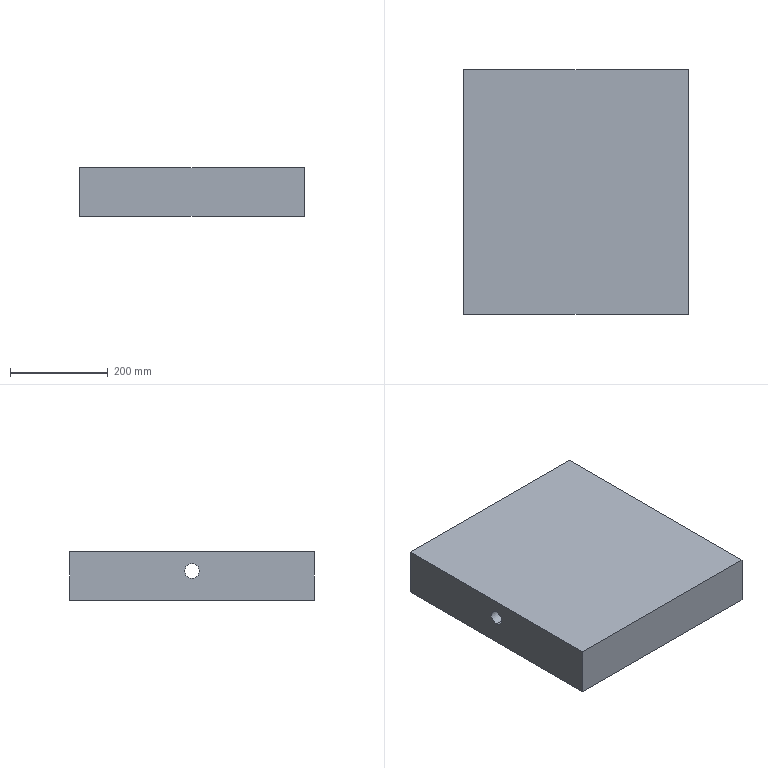Part | SolidWorks | features BaseBody 1, ICE 1 | 1 solid | 13 faces | box 460 x 500 x 100 mm | volume 15946565 mm3 | plane 11 | cylinder 2 | commonest cylinder face diameters 30 x2
STEP:
#1=CARTESIAN_POINT('',(454.836,-175.597,45.));
#2=VERTEX_POINT('',#1);
#3=CARTESIAN_POINT('',(454.836,-175.597,75.));
#4=VERTEX_POINT('',#3);
#5=CARTESIAN_POINT('',(454.836,-175.597,60.));
#6=DIRECTION('',(-1.,0.,0.));
#7=DIRECTION('',(0.,0.,1.));
#8=AXIS2_PLACEMENT_3D('',#5,#6,#7);
#9=CIRCLE('',#8,15.);
#10=EDGE_CURVE('',#2,#4,#9,.T.);
#11=ORIENTED_EDGE('',*,*,#10,.F.);
#12=CARTESIAN_POINT('',(-5.164,-175.597,45.));
#13=VERTEX_POINT('',#12);
#14=CARTESIAN_POINT('',(454.836,-175.597,45.));
#15=DIRECTION('',(-1.,0.,0.));
#16=VECTOR('',#15,1000.);
#17=LINE('',#14,#16);
#18=EDGE_CURVE('',#2,#13,#17,.T.);
#19=ORIENTED_EDGE('',*,*,#18,.T.);
#20=CARTESIAN_POINT('',(-5.164,-175.597,75.));
#21=VERTEX_POINT('',#20);
#22=CARTESIAN_POINT('',(-5.164,-175.597,60.));
#23=DIRECTION('',(-1.,0.,0.));
#24=DIRECTION('',(0.,0.,1.));
#25=AXIS2_PLACEMENT_3D('',#22,#23,#24);
#26=CIRCLE('',#25,15.);
#27=EDGE_CURVE('',#13,#21,#26,.T.);
#28=ORIENTED_EDGE('',*,*,#27,.T.);
#29=CARTESIAN_POINT('',(454.836,-175.597,75.));
#30=DIRECTION('',(-1.,0.,0.));
#31=VECTOR('',#30,1000.);
#32=LINE('',#29,#31);
#33=EDGE_CURVE('',#4,#21,#32,.T.);
#34=ORIENTED_EDGE('',*,*,#33,.F.);
#35=EDGE_LOOP('',(#11,#19,#28,#34));
#36=FACE_OUTER_BOUND('',#35,.T.);
#37=CARTESIAN_POINT('',(454.836,-175.597,60.));
#38=DIRECTION('',(-1.,0.,0.));
#39=DIRECTION('',(0.,0.,1.));
#40=AXIS2_PLACEMENT_3D('',#37,#38,#39);
#41=CYLINDRICAL_SURFACE('',#40,15.);
#42=ADVANCED_FACE('',(#36),#41,.F.);
#43=CARTESIAN_POINT('',(454.836,-425.597,100.));
#44=VERTEX_POINT('',#43);
#45=CARTESIAN_POINT('',(454.836,74.403,100.));
#46=VERTEX_POINT('',#45);
#47=CARTESIAN_POINT('',(454.836,0.,100.));
#48=DIRECTION('',(0.,1.,0.));
#49=VECTOR('',#48,1000.);
#50=LINE('',#47,#49);
#51=EDGE_CURVE('',#44,#46,#50,.T.);
#52=ORIENTED_EDGE('',*,*,#51,.T.);
#53=CARTESIAN_POINT('',(-5.164,74.403,100.));
#54=VERTEX_POINT('',#53);
#55=CARTESIAN_POINT('',(0.,74.403,100.));
#56=DIRECTION('',(-1.,0.,0.));
#57=VECTOR('',#56,1000.);
#58=LINE('',#55,#57);
#59=EDGE_CURVE('',#46,#54,#58,.T.);
#60=ORIENTED_EDGE('',*,*,#59,.T.);
#61=CARTESIAN_POINT('',(-5.164,-425.597,100.));
#62=VERTEX_POINT('',#61);
#63=CARTESIAN_POINT('',(-5.164,0.,100.));
#64=DIRECTION('',(0.,-1.,0.));
#65=VECTOR('',#64,1000.);
#66=LINE('',#63,#65);
#67=EDGE_CURVE('',#54,#62,#66,.T.);
#68=ORIENTED_EDGE('',*,*,#67,.T.);
#69=CARTESIAN_POINT('',(0.,-425.597,100.));
#70=DIRECTION('',(1.,0.,0.));
#71=VECTOR('',#70,1000.);
#72=LINE('',#69,#71);
#73=EDGE_CURVE('',#62,#44,#72,.T.);
#74=ORIENTED_EDGE('',*,*,#73,.T.);
#75=EDGE_LOOP('',(#52,#60,#68,#74));
#76=FACE_OUTER_BOUND('',#75,.T.);
#77=CARTESIAN_POINT('',(0.,0.,100.));
#78=DIRECTION('',(0.,0.,1.));
#79=DIRECTION('',(1.,0.,0.));
#80=AXIS2_PLACEMENT_3D('',#77,#78,#79);
#81=PLANE('',#80);
#82=ADVANCED_FACE('',(#76),#81,.T.);
#83=CARTESIAN_POINT('',(-5.164,74.403,0.));
#84=VERTEX_POINT('',#83);
#85=CARTESIAN_POINT('',(-5.164,74.403,100.));
#86=DIRECTION('',(0.,0.,-1.));
#87=VECTOR('',#86,1000.);
#88=LINE('',#85,#87);
#89=EDGE_CURVE('',#54,#84,#88,.T.);
#90=ORIENTED_EDGE('',*,*,#89,.F.);
#91=ORIENTED_EDGE('',*,*,#59,.F.);
#92=CARTESIAN_POINT('',(454.836,74.403,0.));
#93=VERTEX_POINT('',#92);
#94=CARTESIAN_POINT('',(454.836,74.403,100.));
#95=DIRECTION('',(0.,0.,1.));
#96=VECTOR('',#95,1000.);
#97=LINE('',#94,#96);
#98=EDGE_CURVE('',#93,#46,#97,.T.);
#99=ORIENTED_EDGE('',*,*,#98,.F.);
#100=CARTESIAN_POINT('',(-5.164,74.403,0.));
#101=DIRECTION('',(1.,0.,0.));
#102=VECTOR('',#101,1000.);
#103=LINE('',#100,#102);
#104=EDGE_CURVE('',#84,#93,#103,.T.);
#105=ORIENTED_EDGE('',*,*,#104,.F.);
#106=EDGE_LOOP('',(#90,#91,#99,#105));
#107=FACE_OUTER_BOUND('',#106,.T.);
#108=CARTESIAN_POINT('',(-5.164,74.403,100.));
#109=DIRECTION('',(0.,-1.,0.));
#110=DIRECTION('',(0.,0.,-1.));
#111=AXIS2_PLACEMENT_3D('',#108,#109,#110);
#112=PLANE('',#111);
#113=ADVANCED_FACE('',(#107),#112,.F.);
#114=CARTESIAN_POINT('',(454.836,-175.597,60.));
#115=DIRECTION('',(-1.,0.,0.));
#116=DIRECTION('',(0.,0.,1.));
#117=AXIS2_PLACEMENT_3D('',#114,#115,#116);
#118=CIRCLE('',#117,15.);
#119=EDGE_CURVE('',#4,#2,#118,.T.);
#120=ORIENTED_EDGE('',*,*,#119,.T.);
#121=ORIENTED_EDGE('',*,*,#10,.T.);
#122=EDGE_LOOP('',(#120,#121));
#123=FACE_BOUND('',#122,.T.);
#124=ORIENTED_EDGE('',*,*,#98,.T.);
#125=ORIENTED_EDGE('',*,*,#51,.F.);
#126=CARTESIAN_POINT('',(454.836,-425.597,0.));
#127=VERTEX_POINT('',#126);
#128=CARTESIAN_POINT('',(454.836,-425.597,100.));
#129=DIRECTION('',(0.,0.,1.));
#130=VECTOR('',#129,1000.);
#131=LINE('',#128,#130);
#132=EDGE_CURVE('',#127,#44,#131,.T.);
#133=ORIENTED_EDGE('',*,*,#132,.F.);
#134=CARTESIAN_POINT('',(454.836,74.403,0.));
#135=DIRECTION('',(0.,-1.,0.));
#136=VECTOR('',#135,1000.);
#137=LINE('',#134,#136);
#138=EDGE_CURVE('',#93,#127,#137,.T.);
#139=ORIENTED_EDGE('',*,*,#138,.F.);
#140=EDGE_LOOP('',(#124,#125,#133,#139));
#141=FACE_OUTER_BOUND('',#140,.T.);
#142=CARTESIAN_POINT('',(454.836,74.403,100.));
#143=DIRECTION('',(-1.,0.,0.));
#144=DIRECTION('',(0.,0.,1.));
#145=AXIS2_PLACEMENT_3D('',#142,#143,#144);
#146=PLANE('',#145);
#147=ADVANCED_FACE('',(#123,#141),#146,.F.);
#148=ORIENTED_EDGE('',*,*,#132,.T.);
#149=ORIENTED_EDGE('',*,*,#73,.F.);
#150=CARTESIAN_POINT('',(-5.164,-425.597,0.));
#151=VERTEX_POINT('',#150);
#152=CARTESIAN_POINT('',(-5.164,-425.597,100.));
#153=DIRECTION('',(0.,0.,1.));
#154=VECTOR('',#153,1000.);
#155=LINE('',#152,#154);
#156=EDGE_CURVE('',#151,#62,#155,.T.);
#157=ORIENTED_EDGE('',*,*,#156,.F.);
#158=CARTESIAN_POINT('',(-5.164,-425.597,0.));
#159=DIRECTION('',(-1.,0.,0.));
#160=VECTOR('',#159,1000.);
#161=LINE('',#158,#160);
#162=EDGE_CURVE('',#127,#151,#161,.T.);
#163=ORIENTED_EDGE('',*,*,#162,.F.);
#164=EDGE_LOOP('',(#148,#149,#157,#163));
#165=FACE_OUTER_BOUND('',#164,.T.);
#166=CARTESIAN_POINT('',(-5.164,-425.597,100.));
#167=DIRECTION('',(0.,1.,0.));
#168=DIRECTION('',(0.,0.,1.));
#169=AXIS2_PLACEMENT_3D('',#166,#167,#168);
#170=PLANE('',#169);
#171=ADVANCED_FACE('',(#165),#170,.F.);
#172=CARTESIAN_POINT('',(-5.164,-175.597,60.));
#173=DIRECTION('',(-1.,0.,0.));
#174=DIRECTION('',(0.,0.,1.));
#175=AXIS2_PLACEMENT_3D('',#172,#173,#174);
#176=CIRCLE('',#175,15.);
#177=EDGE_CURVE('',#21,#13,#176,.T.);
#178=ORIENTED_EDGE('',*,*,#177,.F.);
#179=ORIENTED_EDGE('',*,*,#27,.F.);
#180=EDGE_LOOP('',(#178,#179));
#181=FACE_BOUND('',#180,.T.);
#182=ORIENTED_EDGE('',*,*,#156,.T.);
#183=ORIENTED_EDGE('',*,*,#67,.F.);
#184=ORIENTED_EDGE('',*,*,#89,.T.);
#185=CARTESIAN_POINT('',(-5.164,74.403,0.));
#186=DIRECTION('',(0.,1.,0.));
#187=VECTOR('',#186,1000.);
#188=LINE('',#185,#187);
#189=EDGE_CURVE('',#151,#84,#188,.T.);
#190=ORIENTED_EDGE('',*,*,#189,.F.);
#191=EDGE_LOOP('',(#182,#183,#184,#190));
#192=FACE_OUTER_BOUND('',#191,.T.);
#193=CARTESIAN_POINT('',(-5.164,74.403,100.));
#194=DIRECTION('',(1.,0.,0.));
#195=DIRECTION('',(0.,0.,-1.));
#196=AXIS2_PLACEMENT_3D('',#193,#194,#195);
#197=PLANE('',#196);
#198=ADVANCED_FACE('',(#181,#192),#197,.F.);
#199=ORIENTED_EDGE('',*,*,#104,.T.);
#200=ORIENTED_EDGE('',*,*,#138,.T.);
#201=ORIENTED_EDGE('',*,*,#162,.T.);
#202=ORIENTED_EDGE('',*,*,#189,.T.);
#203=EDGE_LOOP('',(#199,#200,#201,#202));
#204=FACE_OUTER_BOUND('',#203,.T.);
#205=CARTESIAN_POINT('',(451.836,-422.597,0.));
#206=VERTEX_POINT('',#205);
#207=CARTESIAN_POINT('',(-2.164,-422.597,0.));
#208=VERTEX_POINT('',#207);
#209=CARTESIAN_POINT('',(0.,-422.597,0.));
#210=DIRECTION('',(-1.,0.,0.));
#211=VECTOR('',#210,1000.);
#212=LINE('',#209,#211);
#213=EDGE_CURVE('',#206,#208,#212,.T.);
#214=ORIENTED_EDGE('',*,*,#213,.F.);
#215=CARTESIAN_POINT('',(451.836,71.403,0.));
#216=VERTEX_POINT('',#215);
#217=CARTESIAN_POINT('',(451.836,0.,0.));
#218=DIRECTION('',(0.,-1.,0.));
#219=VECTOR('',#218,1000.);
#220=LINE('',#217,#219);
#221=EDGE_CURVE('',#216,#206,#220,.T.);
#222=ORIENTED_EDGE('',*,*,#221,.F.);
#223=CARTESIAN_POINT('',(-2.164,71.403,0.));
#224=VERTEX_POINT('',#223);
#225=CARTESIAN_POINT('',(0.,71.403,0.));
#226=DIRECTION('',(1.,0.,0.));
#227=VECTOR('',#226,1000.);
#228=LINE('',#225,#227);
#229=EDGE_CURVE('',#224,#216,#228,.T.);
#230=ORIENTED_EDGE('',*,*,#229,.F.);
#231=CARTESIAN_POINT('',(-2.164,0.,0.));
#232=DIRECTION('',(0.,1.,0.));
#233=VECTOR('',#232,1000.);
#234=LINE('',#231,#233);
#235=EDGE_CURVE('',#208,#224,#234,.T.);
#236=ORIENTED_EDGE('',*,*,#235,.F.);
#237=EDGE_LOOP('',(#214,#222,#230,#236));
#238=FACE_BOUND('',#237,.T.);
#239=CARTESIAN_POINT('',(0.,0.,0.));
#240=DIRECTION('',(0.,0.,1.));
#241=DIRECTION('',(1.,0.,0.));
#242=AXIS2_PLACEMENT_3D('',#239,#240,#241);
#243=PLANE('',#242);
#244=ADVANCED_FACE('',(#204,#238),#243,.F.);
#245=CARTESIAN_POINT('',(-2.164,71.403,30.));
#246=VERTEX_POINT('',#245);
#247=CARTESIAN_POINT('',(-2.164,71.403,30.));
#248=DIRECTION('',(0.,0.,-1.));
#249=VECTOR('',#248,1000.);
#250=LINE('',#247,#249);
#251=EDGE_CURVE('',#246,#224,#250,.T.);
#252=ORIENTED_EDGE('',*,*,#251,.F.);
#253=CARTESIAN_POINT('',(-2.164,-422.597,30.));
#254=VERTEX_POINT('',#253);
#255=CARTESIAN_POINT('',(-2.164,-422.597,30.));
#256=DIRECTION('',(0.,1.,0.));
#257=VECTOR('',#256,1000.);
#258=LINE('',#255,#257);
#259=EDGE_CURVE('',#254,#246,#258,.T.);
#260=ORIENTED_EDGE('',*,*,#259,.F.);
#261=CARTESIAN_POINT('',(-2.164,-422.597,30.));
#262=DIRECTION('',(0.,0.,1.));
#263=VECTOR('',#262,1000.);
#264=LINE('',#261,#263);
#265=EDGE_CURVE('',#208,#254,#264,.T.);
#266=ORIENTED_EDGE('',*,*,#265,.F.);
#267=ORIENTED_EDGE('',*,*,#235,.T.);
#268=EDGE_LOOP('',(#252,#260,#266,#267));
#269=FACE_OUTER_BOUND('',#268,.T.);
#270=CARTESIAN_POINT('',(-2.164,-422.597,30.));
#271=DIRECTION('',(-1.,0.,0.));
#272=DIRECTION('',(0.,0.,1.));
#273=AXIS2_PLACEMENT_3D('',#270,#271,#272);
#274=PLANE('',#273);
#275=ADVANCED_FACE('',(#269),#274,.F.);
#276=ORIENTED_EDGE('',*,*,#265,.T.);
#277=CARTESIAN_POINT('',(451.836,-422.597,30.));
#278=VERTEX_POINT('',#277);
#279=CARTESIAN_POINT('',(451.836,-422.597,30.));
#280=DIRECTION('',(-1.,0.,0.));
#281=VECTOR('',#280,1000.);
#282=LINE('',#279,#281);
#283=EDGE_CURVE('',#278,#254,#282,.T.);
#284=ORIENTED_EDGE('',*,*,#283,.F.);
#285=CARTESIAN_POINT('',(451.836,-422.597,30.));
#286=DIRECTION('',(0.,0.,1.));
#287=VECTOR('',#286,1000.);
#288=LINE('',#285,#287);
#289=EDGE_CURVE('',#206,#278,#288,.T.);
#290=ORIENTED_EDGE('',*,*,#289,.F.);
#291=ORIENTED_EDGE('',*,*,#213,.T.);
#292=EDGE_LOOP('',(#276,#284,#290,#291));
#293=FACE_OUTER_BOUND('',#292,.T.);
#294=CARTESIAN_POINT('',(451.836,-422.597,30.));
#295=DIRECTION('',(0.,-1.,0.));
#296=DIRECTION('',(0.,0.,-1.));
#297=AXIS2_PLACEMENT_3D('',#294,#295,#296);
#298=PLANE('',#297);
#299=ADVANCED_FACE('',(#293),#298,.F.);
#300=ORIENTED_EDGE('',*,*,#289,.T.);
#301=CARTESIAN_POINT('',(451.836,71.403,30.));
#302=VERTEX_POINT('',#301);
#303=CARTESIAN_POINT('',(451.836,71.403,30.));
#304=DIRECTION('',(0.,-1.,0.));
#305=VECTOR('',#304,1000.);
#306=LINE('',#303,#305);
#307=EDGE_CURVE('',#302,#278,#306,.T.);
#308=ORIENTED_EDGE('',*,*,#307,.F.);
#309=CARTESIAN_POINT('',(451.836,71.403,30.));
#310=DIRECTION('',(0.,0.,1.));
#311=VECTOR('',#310,1000.);
#312=LINE('',#309,#311);
#313=EDGE_CURVE('',#216,#302,#312,.T.);
#314=ORIENTED_EDGE('',*,*,#313,.F.);
#315=ORIENTED_EDGE('',*,*,#221,.T.);
#316=EDGE_LOOP('',(#300,#308,#314,#315));
#317=FACE_OUTER_BOUND('',#316,.T.);
#318=CARTESIAN_POINT('',(451.836,71.403,30.));
#319=DIRECTION('',(1.,0.,0.));
#320=DIRECTION('',(0.,0.,-1.));
#321=AXIS2_PLACEMENT_3D('',#318,#319,#320);
#322=PLANE('',#321);
#323=ADVANCED_FACE('',(#317),#322,.F.);
#324=ORIENTED_EDGE('',*,*,#313,.T.);
#325=CARTESIAN_POINT('',(-2.164,71.403,30.));
#326=DIRECTION('',(1.,0.,0.));
#327=VECTOR('',#326,1000.);
#328=LINE('',#325,#327);
#329=EDGE_CURVE('',#246,#302,#328,.T.);
#330=ORIENTED_EDGE('',*,*,#329,.F.);
#331=ORIENTED_EDGE('',*,*,#251,.T.);
#332=ORIENTED_EDGE('',*,*,#229,.T.);
#333=EDGE_LOOP('',(#324,#330,#331,#332));
#334=FACE_OUTER_BOUND('',#333,.T.);
#335=CARTESIAN_POINT('',(-2.164,71.403,30.));
#336=DIRECTION('',(0.,1.,0.));
#337=DIRECTION('',(0.,0.,1.));
#338=AXIS2_PLACEMENT_3D('',#335,#336,#337);
#339=PLANE('',#338);
#340=ADVANCED_FACE('',(#334),#339,.F.);
#341=ORIENTED_EDGE('',*,*,#329,.T.);
#342=ORIENTED_EDGE('',*,*,#307,.T.);
#343=ORIENTED_EDGE('',*,*,#283,.T.);
#344=ORIENTED_EDGE('',*,*,#259,.T.);
#345=EDGE_LOOP('',(#341,#342,#343,#344));
#346=FACE_OUTER_BOUND('',#345,.T.);
#347=CARTESIAN_POINT('',(0.,0.,30.));
#348=DIRECTION('',(0.,0.,-1.));
#349=DIRECTION('',(-1.,0.,0.));
#350=AXIS2_PLACEMENT_3D('',#347,#348,#349);
#351=PLANE('',#350);
#352=ADVANCED_FACE('',(#346),#351,.T.);
#353=ORIENTED_EDGE('',*,*,#18,.F.);
#354=ORIENTED_EDGE('',*,*,#119,.F.);
#355=ORIENTED_EDGE('',*,*,#33,.T.);
#356=ORIENTED_EDGE('',*,*,#177,.T.);
#357=EDGE_LOOP('',(#353,#354,#355,#356));
#358=FACE_OUTER_BOUND('',#357,.T.);
#359=CARTESIAN_POINT('',(454.836,-175.597,60.));
#360=DIRECTION('',(-1.,0.,0.));
#361=DIRECTION('',(0.,0.,1.));
#362=AXIS2_PLACEMENT_3D('',#359,#360,#361);
#363=CYLINDRICAL_SURFACE('',#362,15.);
#364=ADVANCED_FACE('',(#358),#363,.F.);
#365=CLOSED_SHELL('',(#42,#82,#113,#147,#171,#198,#244,#275,#299,#323,#340,#352,#364));
#366=MANIFOLD_SOLID_BREP('',#365);
#367=CARTESIAN_POINT('',(0.,0.,0.));
#368=DIRECTION('',(0.,0.,1.));
#369=DIRECTION('',(1.,0.,0.));
#370=AXIS2_PLACEMENT_3D('',#367,#368,#369);
#371=(LENGTH_UNIT()NAMED_UNIT(*)SI_UNIT(.MILLI.,.METRE.));
#372=UNCERTAINTY_MEASURE_WITH_UNIT(LENGTH_MEASURE(0.00001),#371,'','');
#373=(NAMED_UNIT(*)PLANE_ANGLE_UNIT()SI_UNIT($,.RADIAN.));
#374=(NAMED_UNIT(*)SI_UNIT($,.STERADIAN.)SOLID_ANGLE_UNIT());
#375=(GEOMETRIC_REPRESENTATION_CONTEXT(3)GLOBAL_UNCERTAINTY_ASSIGNED_CONTEXT((#372))GLOBAL_UNIT_ASSIGNED_CONTEXT((#371,#373,#374))REPRESENTATION_CONTEXT('',''));
#376=ADVANCED_BREP_SHAPE_REPRESENTATION('',(#366,#370),#375);